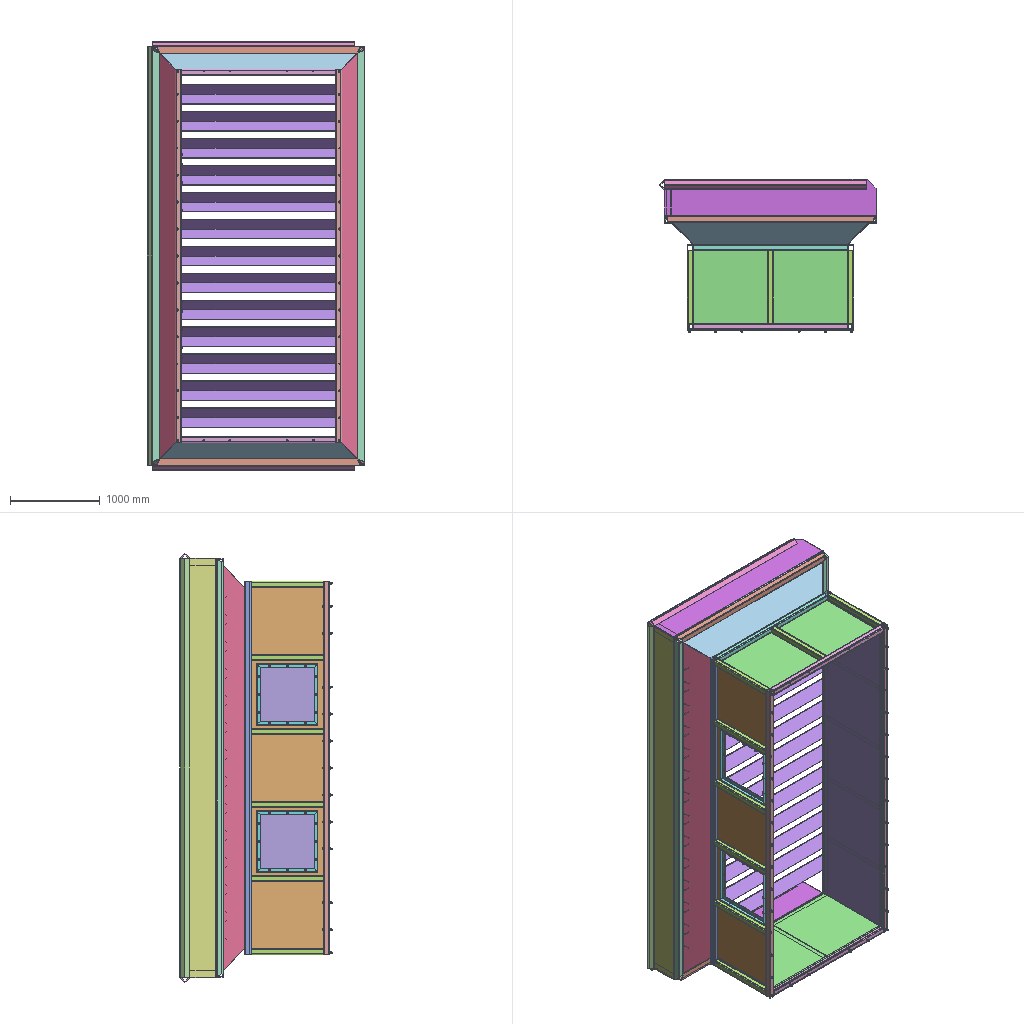Assembly | SolidWorks | 26 different items | 306 placed | box 2415 x 1700 x 4774 mm
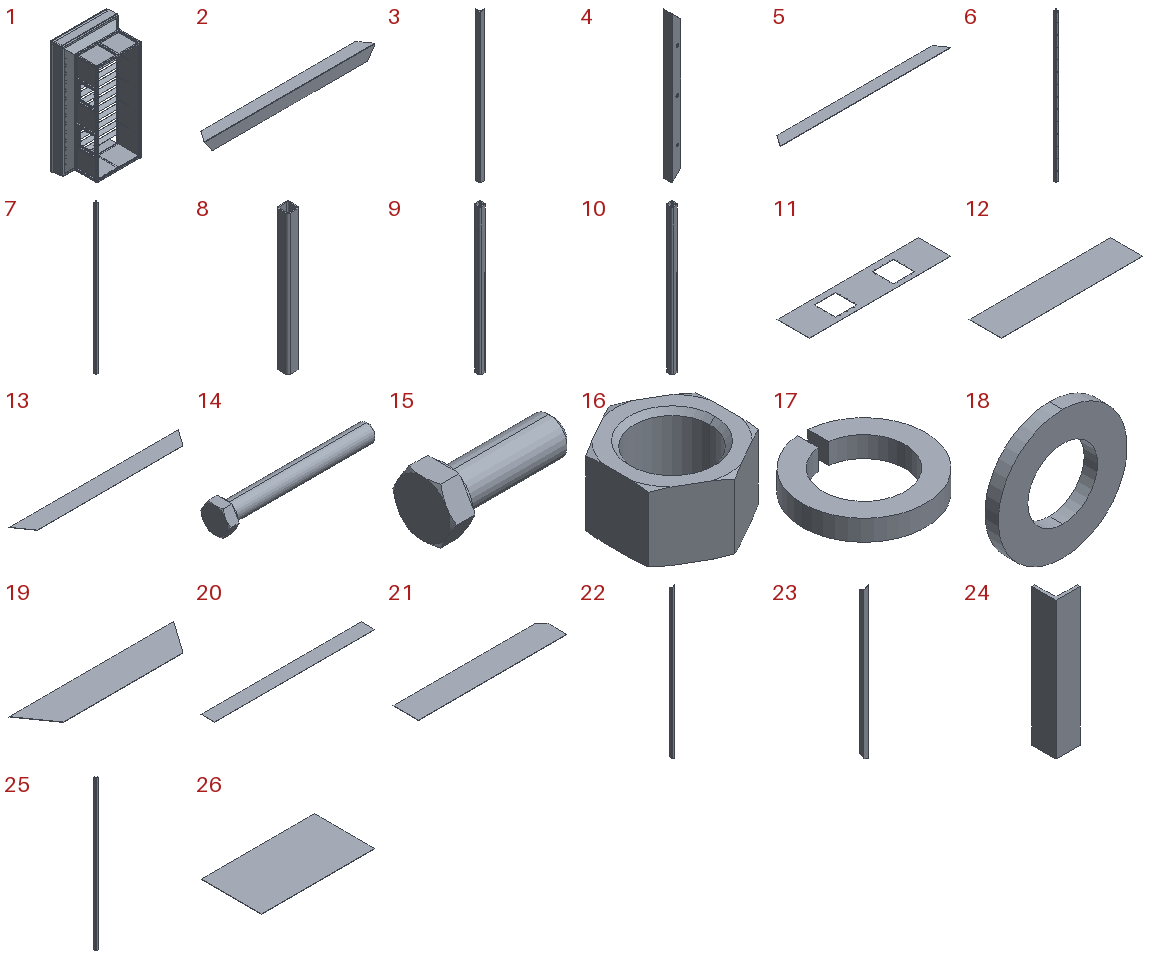Parts list (item | name | quantity | parent item | size | volume | features):
1 | (subassembly) | x1 | - | 2415 x 1670 x 4774 mm | 225195392 mm3 | features ReferencePattern 53, LocalLPattern 8, MirrorCompFeat 3
2 | (subassembly) | x13 | in 1 | 2328 x 156 x 156 mm | 4001344 mm3 | -
3 | - | x2 | in 1 | 70 x 70 x 2250 mm | 2398211 mm3 | features Extrusion 1
4 | - | x8 | in 1 | 40 x 40 x 680 mm | 199359 mm3 | features ICE 2, Extrusion 1
5 | - | x26 | in 2 | 2328 x 150 x 6 mm | 2000672 mm3 | features FlatPattern 1, SMBaseFlange 1, SheetMetal 1
6 | - | x2 | in 1 | 70 x 70 x 4160 mm | 5980203 mm3 | features ICE 2, Extrusion 1
7 | - | x2 | in 1 | 70 x 70 x 4160 mm | 6004095 mm3 | features Extrusion 1
8 | - | x14 | in 1 | 70 x 70 x 805 mm | 1161850 mm3 | features Extrusion 1
9 | - | x2 | in 1 | 70 x 70 x 1716 mm | 2470318 mm3 | features Extrusion 1, ICE 1, LPattern 1
10 | - | x2 | in 1 | 70 x 70 x 1716 mm | 2476689 mm3 | features Extrusion 1
11 | - | x1 | in 1 | 4020 x 910 x 5 mm | 14675072 mm3 | features ICE 2, FlatPattern 1, LPattern 1, SMBaseFlange 1, SheetMetal 1
12 | - | x1 | in 1 | 4020 x 910 x 5 mm | 18291000 mm3 | features FlatPattern 1, SMBaseFlange 1, SheetMetal 1
13 | - | x2 | in 1 | 4660 x 455 x 5 mm | 9873500 mm3 | features FlatPattern 1, SMBaseFlange 1, SheetMetal 1
14 | - | x26 | - | 107.5 x 20.785 x 18 mm | 13361 mm3 | features RevCut 4, Chamfer 1, Extrusion 1, Fillet 1, LPattern 1, Revolution 1
15 | - | x28 | in 1 | 42.5 x 20.785 x 18 mm | 6010 mm3 | features RevCut 4, Chamfer 1, Extrusion 1, Fillet 1, LPattern 1, Revolution 1
16 | - | x54 | - | 17.386 x 20.03 x 10.8 mm | 1566 mm3 | features Cut 2, Chamfer 1, Extrusion 1
17 | - | x54 | - | 18.367 x 18.334 x 3.1 mm | 444.091 mm3 | features Extrusion 1
18 | - | x54 | - | 24 x 2.5 x 24 mm | 799.143 mm3 | features Revolution 1
19 | - | x2 | in 1 | 2348 x 455 x 5 mm | 4611425 mm3 | features FlatPattern 1, SMBaseFlange 1, SheetMetal 1
20 | - | x1 | in 1 | 4660 x 400 x 5 mm | 9320000 mm3 | features FlatPattern 1, SMBaseFlange 1, SheetMetal 1
21 | - | x2 | in 1 | 2350 x 400 x 5 mm | 4675000 mm3 | features FlatPattern 1, SMBaseFlange 1, SheetMetal 1
22 | - | x2 | in 1 | 70 x 70 x 4645 mm | 4877091 mm3 | features Extrusion 1, ICE 1
23 | - | x2 | in 1 | 70 x 70 x 2334 mm | 2413861 mm3 | features Extrusion 1, ICE 1
24 | - | x2 | in 1 | 70 x 70 x 400 mm | 426349 mm3 | features Extrusion 1
25 | - | x1 | in 1 | 70 x 70 x 4660 mm | 4966962 mm3 | features Extrusion 1
26 | - | x2 | in 1 | 1704 x 910 x 5 mm | 7753200 mm3 | features FlatPattern 1, SMBaseFlange 1, SheetMetal 1
Mates (type | each side: item.copy, entity, surface, feature):
In the top assembly
Coincident | 4.1 face plane Boss-Extrude1 | assembly face
Concentric | assembly face | 15.1 face cylinder Boss-Revolve1
Parallel | 4.2 face plane Boss-Extrude1 | assembly face
Concentric | 17.1 face cylinder Extrude1 | 18.1 face cylinder Base-revolve
Coincident | 17.1 face plane Extrude1 | 18.1 face plane Base-revolve
Coincident | 16.1 face plane Base-extrude | 17.1 face plane Extrude1
Concentric | 16.1 face cylinder Base-extrude | 17.1 face cylinder Extrude1
Concentric | 15.2 face cylinder Boss-Revolve1 | 16.1 face cylinder Base-extrude
Coincident | assembly face | 18.1 face plane Base-revolve
Concentric | 17.2 face cylinder Extrude1 | 18.2 face cylinder Base-revolve
Coincident | 18.2 face plane Base-revolve | 17.2 face plane Extrude1
Coincident | 17.2 face plane Extrude1 | 16.2 face plane Base-extrude
Concentric | 18.2 face cylinder Base-revolve | 16.2 face cylinder Base-extrude
Concentric | 15.3 face cylinder Boss-Revolve1 | 16.2 face cylinder Base-extrude
Coincident | assembly face | 18.2 face plane Base-revolve
Concentric | 15.4 face cylinder Boss-Revolve1 | 18.3 face cylinder Base-revolve
Concentric | 18.3 face cylinder Base-revolve | 17.3 face cylinder Extrude1
Coincident | 17.3 face plane Extrude1 | 18.3 face plane Base-revolve
Coincident | 16.3 face plane Base-extrude | 17.3 face plane Extrude1
Concentric | 15.4 face cylinder Boss-Revolve1 | 16.3 face cylinder Base-extrude
DistanceDim | 15.4 face plane Base-extrude | 18.3 face plane Base-revolve
Concentric | 6.1 face cylinder Cut-Extrude2 | 15.4 face cylinder Boss-Revolve1
Coincident | 6.1 face plane Boss-Extrude1 | 15.4 face plane Base-extrude
Concentric | 15.5 face cylinder Boss-Revolve1 | 18.4 face cylinder Base-revolve
Concentric | 18.4 face cylinder Base-revolve | 17.4 face cylinder Extrude1
Coincident | 18.4 face plane Base-revolve | 17.4 face plane Extrude1
Coincident | 17.4 face plane Extrude1 | 16.4 face plane Base-extrude
Concentric | 15.5 face cylinder Boss-Revolve1 | 16.4 face cylinder Base-extrude
DistanceDim | 15.5 face plane Base-extrude | 18.4 face plane Base-revolve
Concentric | 6.2 face cylinder Cut-Extrude2 | 15.5 face cylinder Boss-Revolve1
Coincident | 6.2 face plane Boss-Extrude1 | 15.5 face plane Base-extrude
Concentric | 15.6 face cylinder Boss-Revolve1 | 18.5 face cylinder Base-revolve
Concentric | 18.5 face cylinder Base-revolve | 17.5 face cylinder Extrude1
Coincident | 18.5 face plane Base-revolve | 17.5 face plane Extrude1
Coincident | 17.5 face plane Extrude1 | 16.5 face plane Base-extrude
Concentric | 15.6 face cylinder Boss-Revolve1 | 16.5 face cylinder Base-extrude
DistanceDim | 15.6 face plane Base-extrude | 18.5 face plane Base-revolve
Concentric | 6.2 face cylinder Cut-Extrude2 | 15.6 face cylinder Boss-Revolve1
Coincident | 6.2 face plane Boss-Extrude1 | 15.6 face plane Base-extrude
Concentric | 15.7 face cylinder Boss-Revolve1 | 18.6 face cylinder Base-revolve
Concentric | 18.6 face cylinder Base-revolve | 17.6 face cylinder Extrude1
Coincident | 18.6 face plane Base-revolve | 17.6 face plane Extrude1
Coincident | 17.6 face plane Extrude1 | 16.6 face plane Base-extrude
Concentric | 15.7 face cylinder Boss-Revolve1 | 16.6 face cylinder Base-extrude
DistanceDim | 15.7 face plane Base-extrude | 18.6 face plane Base-revolve
Concentric | 6.1 face cylinder Cut-Extrude2 | 15.7 face cylinder Boss-Revolve1
Coincident | 6.1 face plane Boss-Extrude1 | 15.7 face plane Base-extrude
Concentric | 14.1 face cylinder Boss-Revolve1 | 18.7 face cylinder Base-revolve
Concentric | 18.7 face cylinder Base-revolve | 17.7 face cylinder Extrude1
Coincident | 18.7 face plane Base-revolve | 17.7 face plane Extrude1
Coincident | 17.7 face plane Extrude1 | 16.7 face plane Base-extrude
Concentric | 14.1 face cylinder Boss-Revolve1 | 16.7 face cylinder Base-extrude
DistanceDim | 14.1 face plane Base-extrude | 18.7 face plane Base-revolve
Concentric | 9.1 face cylinder Cut-Extrude1 | 14.1 face cylinder Boss-Revolve1
Coincident | 9.1 face plane Boss-Extrude1 | 14.1 face plane Base-extrude
Concentric | 14.2 face cylinder Boss-Revolve1 | 18.8 face cylinder Base-revolve
Concentric | 18.8 face cylinder Base-revolve | 17.8 face cylinder Extrude1
Coincident | 18.8 face plane Base-revolve | 17.8 face plane Extrude1
Coincident | 17.8 face plane Extrude1 | 16.8 face plane Base-extrude
Concentric | 14.2 face cylinder Boss-Revolve1 | 16.8 face cylinder Base-extrude
DistanceDim | 14.2 face plane Base-extrude | 18.8 face plane Base-revolve
Concentric | 9.1 face cylinder Cut-Extrude1 | 14.2 face cylinder Boss-Revolve1
Coincident | 9.1 face plane Boss-Extrude1 | 14.2 face plane Base-extrude
Concentric | 14.3 face cylinder Boss-Revolve1 | 18.9 face cylinder Base-revolve
Concentric | 18.9 face cylinder Base-revolve | 17.9 face cylinder Extrude1
Coincident | 18.9 face plane Base-revolve | 17.9 face plane Extrude1
Coincident | 17.9 face plane Extrude1 | 16.9 face plane Base-extrude
Concentric | 14.3 face cylinder Boss-Revolve1 | 16.9 face cylinder Base-extrude
DistanceDim | 14.3 face plane Base-extrude | 18.9 face plane Base-revolve
Concentric | 6.1 face cylinder Cut-Extrude1 | 14.3 face cylinder Boss-Revolve1
Coincident | 6.1 face plane Boss-Extrude1 | 14.3 face plane Base-extrude
Concentric | assembly face | assembly face | 6 times
Coincident | assembly face | assembly face | 4 times
DistanceDim | assembly face | assembly face | 2 times
Concentric | 9.2 face cylinder Cut-Extrude1 | assembly face | 2 times
Coincident | 9.2 face plane Boss-Extrude1 | assembly face | 3 times
Coincident | 6.2 face plane Boss-Extrude1 | 9.1 face plane Boss-Extrude1
Concentric | assembly face | 17.10 face
Coincident | assembly face | 17.10 face plane Extrude1
DistanceDim | 9.1 face plane Boss-Extrude1 | 18.10 face plane Base-revolve
Concentric | 14.4 face cylinder Boss-Revolve1 | 18.10 face cylinder Base-revolve
Concentric | 18.10 face cylinder Base-revolve | 17.10 face cylinder Extrude1
Coincident | 18.10 face plane Base-revolve | 17.10 face plane Extrude1
Coincident | 17.10 face plane Extrude1 | 16.10 face plane Base-extrude
Concentric | 14.4 face cylinder Boss-Revolve1 | 16.10 face cylinder Base-extrude
Concentric | 9.1 face cylinder LPattern1 | 14.4 face cylinder Boss-Revolve1
Coincident | 9.1 face plane Boss-Extrude1 | 14.4 face plane Base-extrude
Concentric | 14.5 face cylinder Boss-Revolve1 | 18.11 face cylinder Base-revolve
Concentric | 18.11 face cylinder Base-revolve | 17.11 face cylinder Extrude1
Coincident | 18.11 face plane Base-revolve | 17.11 face plane Extrude1
Coincident | 17.11 face plane Extrude1 | 16.11 face plane Base-extrude
Concentric | 14.5 face cylinder Boss-Revolve1 | 16.11 face cylinder Base-extrude
DistanceDim | 14.5 face plane Base-extrude | 18.11 face plane Base-revolve
Concentric | 9.1 face cylinder LPattern1 | 14.5 face cylinder Boss-Revolve1
Coincident | 9.1 face plane Boss-Extrude1 | 14.5 face plane Base-extrude
Concentric | 9.2 face cylinder LPattern1 | assembly face
In subassembly 1
Coincident | 6.3 face plane Boss-Extrude1 | 7.1 face plane Boss-Extrude1 | 2 times
DistanceDim | 7.1 face plane Boss-Extrude1 | 6.3 face plane Boss-Extrude1
Coincident | 6.3 face plane Boss-Extrude1 | 8.1 face plane Boss-Extrude1 | 3 times
Coincident | 6.3 face plane Boss-Extrude1 | 9.3 face plane Boss-Extrude1 | 2 times
Coincident | 7.1 face plane Boss-Extrude1 | 10.1 face plane Boss-Extrude1 | 3 times
Coincident | 7.1 face plane Boss-Extrude1 | 11.1 face plane Base-Flange1 | 2 times
Coincident | 10.1 face plane Boss-Extrude1 | 11.1 face plane Base-Flange1
Coincident | 8.2 face plane Boss-Extrude1 | 12.1 face plane Base-Flange1
Coincident | 7.2 face plane Boss-Extrude1 | 12.1 face plane Base-Flange1
Coincident | 10.1 face plane Boss-Extrude1 | 12.1 face plane Base-Flange1
Coincident | 12.1 face plane Base-Flange1 | 26.1 face plane Base-Flange1
DistanceDim | 26.1 face plane Base-Flange1 | 11.1 face plane Base-Flange1
Coincident | 10.1 face plane Boss-Extrude1 | 26.2 face plane Base-Flange1
Coincident | 11.1 face plane Base-Flange1 | 26.2 face plane Base-Flange1
DistanceDim | 11.1 face plane Base-Flange1 | 26.2 face plane Base-Flange1
Coincident | 8.1 face plane Boss-Extrude1 | 9.3 face plane Boss-Extrude1
Coincident | 1.1 face | 9.4 face plane Boss-Extrude1
Coincident | 6.3 face plane Boss-Extrude1 | 9.4 face plane Boss-Extrude1 | 3 times
Coincident | 7.1 face plane Boss-Extrude1 | 10.2 face plane Boss-Extrude1 | 3 times
Coincident | 9.4 face plane Boss-Extrude1 | 6.4 face plane Boss-Extrude1 | 2 times
Coincident | 8.3 face plane Boss-Extrude1 | 6.4 face plane Boss-Extrude1
Coincident | 12.1 edge | 13.1 edge
PlanarAngleDim | 13.1 face plane Base-Flange1 | 12.1 face plane Base-Flange1
Coincident | 12.1 face plane Base-Flange1 | 13.1 edge
Coincident | 26.1 face plane Base-Flange1 | 10.2 face plane Boss-Extrude1
Coincident | 26.2 edge | 19.1 edge
PlanarAngleDim | 19.1 face plane Base-Flange1 | 26.2 face plane Base-Flange1
DistanceDim | 12.1 face plane Base-Flange1 | 19.1 edge
Coincident | 11.1 edge | 13.2 edge
PlanarAngleDim | 13.2 face plane Base-Flange1 | 11.1 face plane Base-Flange1
Coincident | 11.1 face plane Base-Flange1 | 13.2 edge
Coincident | 26.1 edge | 19.2 edge
PlanarAngleDim | 19.2 face plane Base-Flange1 | 26.1 face plane Base-Flange1
DistanceDim | 11.1 face plane Base-Flange1 | 19.2 edge
Coincident | 13.2 edge | 20.1 edge
PlanarAngleDim | 20.1 face plane Base-Flange1 | 13.2 face plane Base-Flange1
Coincident | 13.2 face plane Base-Flange1 | 20.1 vertex
Coincident | 19.1 edge | 21.1 edge
PlanarAngleDim | 19.1 face plane Base-Flange1 | 21.1 face plane Base-Flange1
Coincident | 20.1 face plane Base-Flange1 | 21.1 vertex
Coincident | 19.2 edge | 21.2 edge
PlanarAngleDim | 21.2 face plane Base-Flange1 | 19.2 face plane Base-Flange1
Coincident | 20.1 face plane Base-Flange1 | 21.2 vertex
DistanceDim | 13.1 face plane Base-Flange1 | 22.1 edge
Tangent | 13.1 face plane Base-Flange1 | 22.1 face cylinder Boss-Extrude1 | 2 times
Coincident | 13.1 vertex | 22.1 face plane Cut-Extrude4
Tangent | 19.2 face plane Base-Flange1 | 23.1 face cylinder Boss-Extrude1 | 2 times
DistanceDim | 23.1 edge | 19.2 face plane Base-Flange1
Coincident | 19.2 vertex | 23.1 face plane Cut-Extrude4
Coincident | 20.1 face plane Base-Flange1 | 24.1 face plane Boss-Extrude1 | 2 times
Coincident | 21.1 face plane Base-Flange1 | 24.1 vertex
Coincident | 20.1 face plane Base-Flange1 | 24.2 face plane Boss-Extrude1 | 2 times
Coincident | 21.2 face plane Base-Flange1 | 24.2 vertex
Coincident | 20.1 face plane Base-Flange1 | 25.1 face plane Boss-Extrude1
DistanceDim | 25.1 edge | 20.1 face plane Base-Flange1
DistanceDim | 25.1 plane | 20.1 face plane Base-Flange1
DistanceDim | 3.1 plane | 21.1 face plane Base-Flange1
DistanceDim | 3.1 edge | 21.1 face plane Base-Flange1
Coincident | 20.1 face plane Base-Flange1 | 3.1 vertex
Coincident | 4.3 face plane Cut-Extrude1 | 4.4 face plane Cut-Extrude1
Coincident | 4.3 face plane Boss-Extrude1 | 4.4 face plane Boss-Extrude1
Coincident | 4.3 edge | 4.4 face plane Boss-Extrude1
Coincident | 4.4 face plane Boss-Extrude1 | 4.5 face plane Boss-Extrude1
Coincident | 4.4 face plane Boss-Extrude1 | 4.6 face plane Boss-Extrude1
Coincident | 4.4 face plane Cut-Extrude1 | 4.6 face plane Cut-Extrude1
Coincident | 4.4 edge | 4.6 face plane Boss-Extrude1
Coincident | 4.3 face plane Cut-Extrude1 | 4.5 face plane Cut-Extrude1
Coincident | 4.3 face plane Boss-Extrude1 | 4.5 edge
Coincident | 11.1 face plane Base-Flange1 | 4.5 face plane Boss-Extrude1
Coincident | 11.1 face plane Cut-Extrude1 | 4.3 face plane Boss-Extrude1
Coincident | 11.1 face plane Cut-Extrude1 | 4.5 face plane Boss-Extrude1
Concentric | 11.1 face cylinder LPattern1 | 15.4 face cylinder Boss-Revolve1
Coincident | 11.1 face plane Base-Flange1 | 15.4 face plane Base-extrude
Concentric | 11.1 face cylinder LPattern1 | 15.5 face cylinder Boss-Revolve1
Coincident | 11.1 face plane Base-Flange1 | 15.5 face plane Base-extrude
Coincident | 26.1 face plane Base-Flange1 | 8.4 face plane Boss-Extrude1
Coincident | 10.2 face plane Boss-Extrude1 | 8.4 face plane Boss-Extrude1
DistanceDim | 8.4 face plane Boss-Extrude1 | 8.5 face plane Boss-Extrude1
Coincident | 26.2 face plane Base-Flange1 | 8.6 face plane Boss-Extrude1
DistanceDim | 8.6 face plane Boss-Extrude1 | 8.7 face plane Boss-Extrude1
Coincident | 10.1 face plane Boss-Extrude1 | 8.6 face plane Boss-Extrude1
DistanceDim | 1.1 plane | 10.2 face plane Boss-Extrude1 | 4 times
DistanceDim | 1.1 plane | 7.2 face plane Boss-Extrude1
DistanceDim | 1.1 plane | 23.1 face plane Boss-Extrude1 | 2 times
DistanceDim | 1.1 plane | 23.1 vertex
Coincident | 6.3 face plane Boss-Extrude1 | 1.1 face
Coincident | 26.1 face plane Base-Flange1 | 1.1 face
DistanceDim | 1.1 face | 12.1 face plane Base-Flange1
DistanceDim | 5.1 edge | 6.4 face plane Boss-Extrude1
DistanceDim | 5.2 edge | 6.4 face plane Boss-Extrude1
DistanceDim | 5.2 edge | 26.1 face plane Base-Flange1
Coincident | 13.1 face plane Base-Flange1 | 5.1 vertex
In subassembly 2
Coincident | 5.3 edge | 5.4 edge
PlanarAngleDim | 5.3 face plane Base-Flange1 | 5.4 face plane Base-Flange1
Coincident | 5.3 vertex | 5.4 face plane Base-Flange1